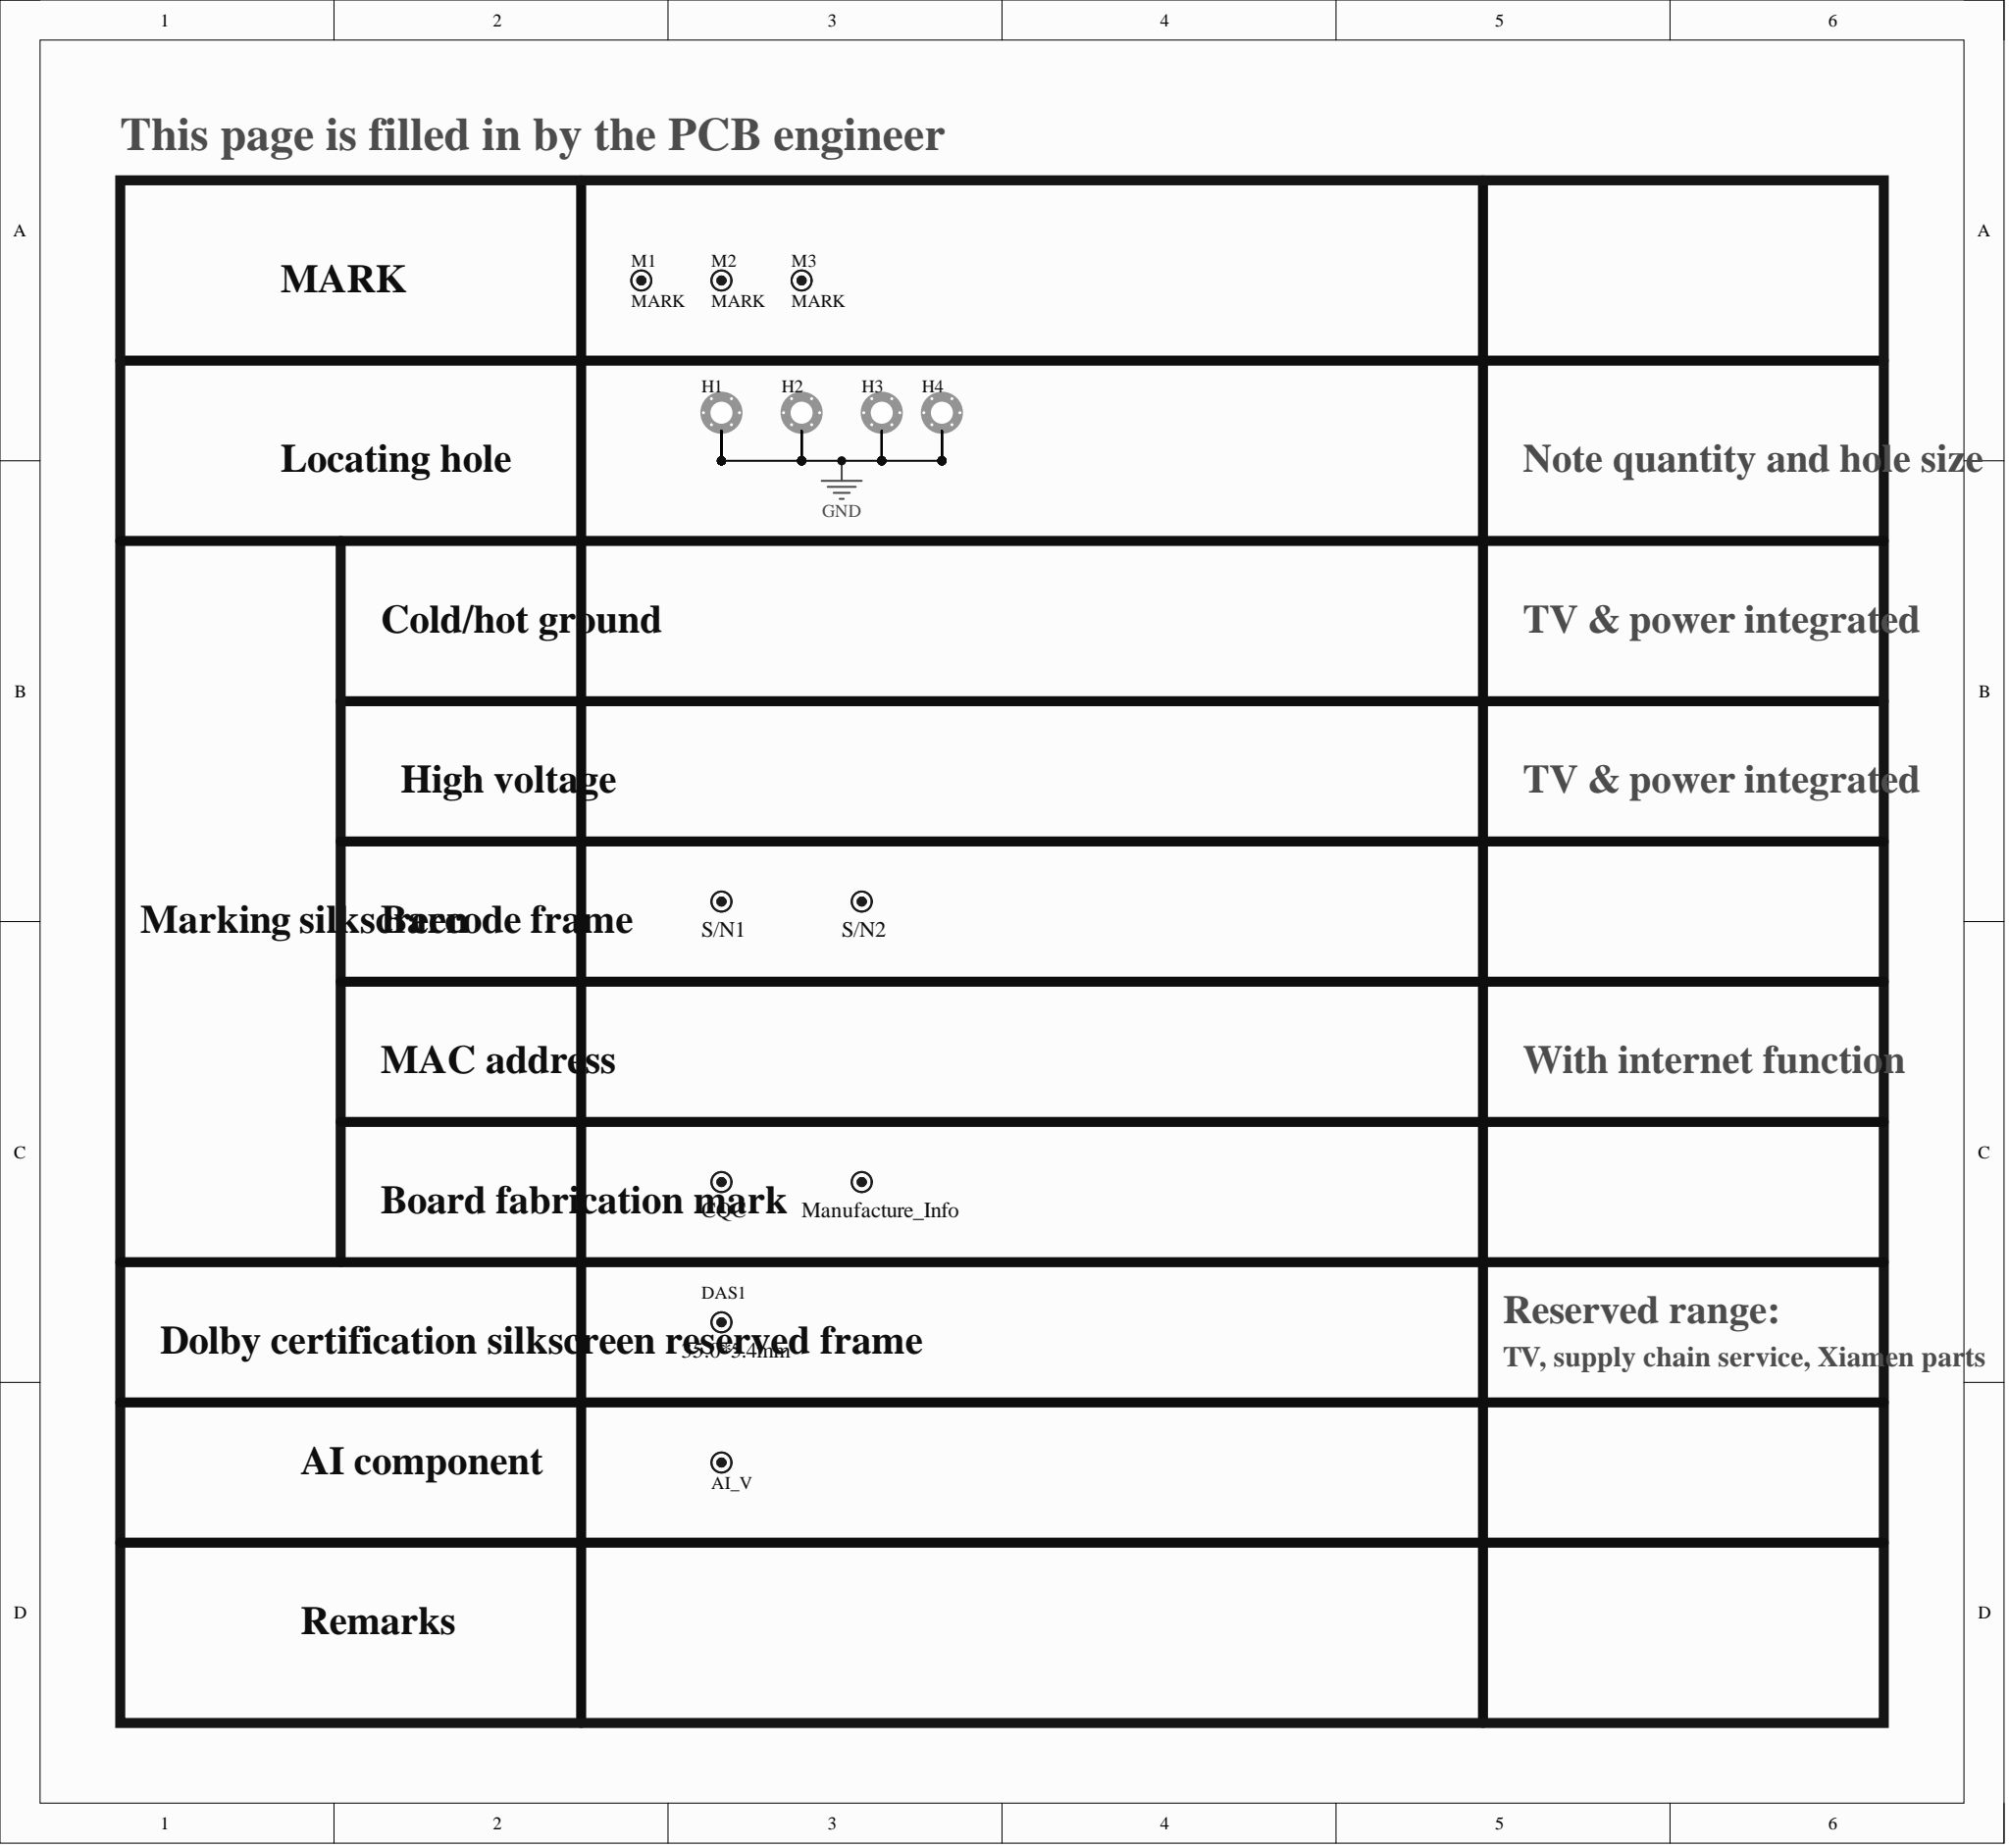Circuit board | Altium Designer | 541 parts | 263 nets | one sheet of the schematic
Parts on this sheet (reference | value | footprint):
AI_V | AI_GRIPPER_V | AI_GRIPPER_V
CQC | CQC | CQC
DAS1 | 35.0*5.4mm | DOLBY_AS2
H1 | Location hole | ASSE4.0C-3
H2 | Location hole | ASSE4.0C-3
H3 | Location hole | ASSE4.0C-3
H4 | Location hole | ASSE4.0C-3
M1 | MARK | MARK
M2 | MARK | MARK
M3 | MARK | MARK
Manufacture_Info | Manufacture_Info | Manufacture_Info
S/N1 | Barcode | Barcode
S/N2 | Barcode | Barcode
Nets of these parts (net: part-pin ...):
GND: H1-1 H1-2 H1-3 H1-4 H1-5 H1-6 H2-1 H2-2 H2-3 H2-4 H2-5 H2-6 H3-1 H3-2 H3-3 H3-4 H3-5 H3-6 H4-1 H4-2 H4-3 H4-4 H4-5 H4-6